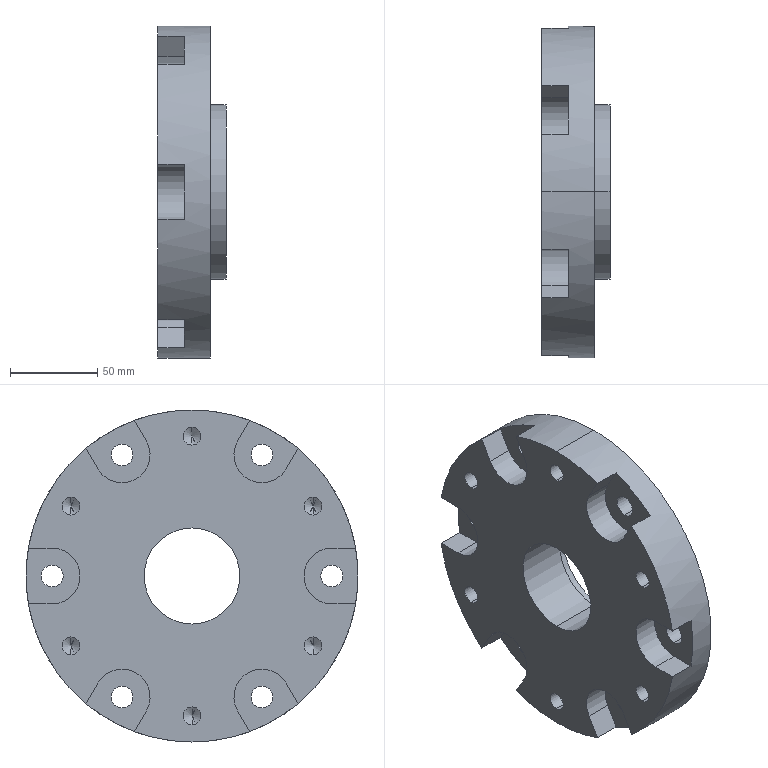Part | SolidWorks | features CirPattern 3, ICE 3, 3DProfileFeature 1, HoleWzd 1, Revolution 1 | 1 solid | 74 faces | box 39 x 190 x 190 mm | volume 716899 mm3 | cylinder 40 | plane 22 | cone 12 | commonest cylinder face diameters 10.2 x12 12.5 x12 32 x8 55 x2 70 x2 100 x2